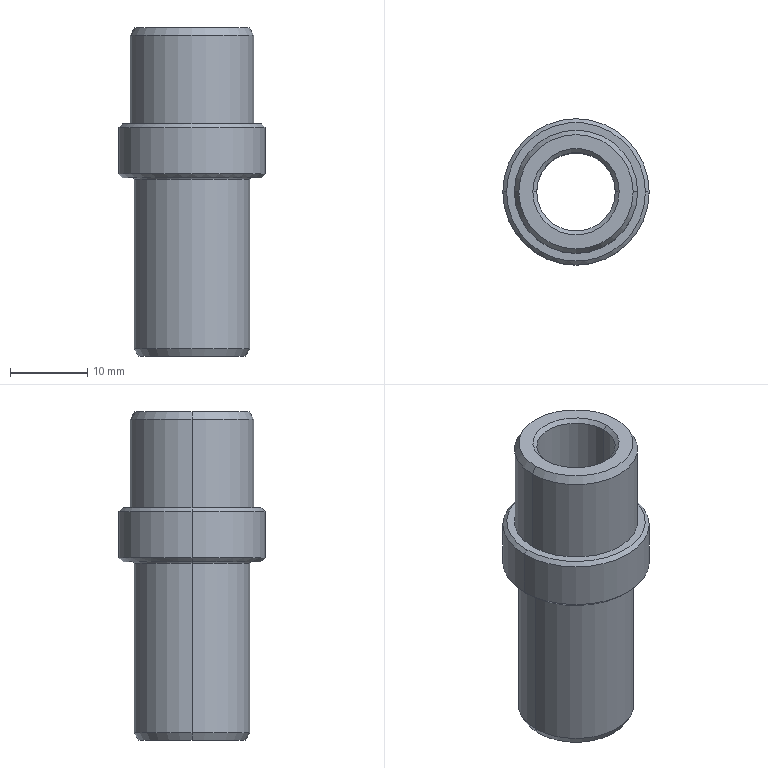Part | STEP file | PERNO RODAJA FRONTAL | 1 solid | 26 faces | box 19 x 19 x 42.7 mm | volume 5059 mm3 | cone 12 | cylinder 8 | plane 4 | torus 2 | commonest cylinder face diameters 10.2 x2 15 x2 16 x2 19 x2
STEP:
#1=CARTESIAN_POINT('',(7.423,0.,10.5));
#2=VERTEX_POINT('',#1);
#3=CARTESIAN_POINT('',(-7.423,0.,10.5));
#4=VERTEX_POINT('',#3);
#5=CARTESIAN_POINT('',(0.,0.,10.5));
#6=DIRECTION('',(0.,0.,1.));
#7=DIRECTION('',(1.,0.,0.));
#8=AXIS2_PLACEMENT_3D('',#5,#6,#7);
#9=CIRCLE('',#8,7.423);
#10=EDGE_CURVE('',#2,#4,#9,.T.);
#11=ORIENTED_EDGE('',*,*,#10,.F.);
#12=CARTESIAN_POINT('',(8.,0.,9.5));
#13=VERTEX_POINT('',#12);
#14=CARTESIAN_POINT('',(7.423,0.,10.5));
#15=DIRECTION('',(0.5,0.,-0.866));
#16=VECTOR('',#15,1000.);
#17=LINE('',#14,#16);
#18=EDGE_CURVE('',#2,#13,#17,.T.);
#19=ORIENTED_EDGE('',*,*,#18,.T.);
#20=CARTESIAN_POINT('',(-8.,0.,9.5));
#21=VERTEX_POINT('',#20);
#22=CARTESIAN_POINT('',(0.,0.,9.5));
#23=DIRECTION('',(0.,0.,-1.));
#24=DIRECTION('',(1.,0.,0.));
#25=AXIS2_PLACEMENT_3D('',#22,#23,#24);
#26=CIRCLE('',#25,8.);
#27=EDGE_CURVE('',#21,#13,#26,.T.);
#28=ORIENTED_EDGE('',*,*,#27,.F.);
#29=CARTESIAN_POINT('',(-7.423,0.,10.5));
#30=DIRECTION('',(-0.5,0.,-0.866));
#31=VECTOR('',#30,1000.);
#32=LINE('',#29,#31);
#33=EDGE_CURVE('',#4,#21,#32,.T.);
#34=ORIENTED_EDGE('',*,*,#33,.F.);
#35=EDGE_LOOP('',(#11,#19,#28,#34));
#36=FACE_OUTER_BOUND('',#35,.T.);
#37=CARTESIAN_POINT('',(0.,0.,10.5));
#38=DIRECTION('',(0.,0.,-1.));
#39=DIRECTION('',(-1.,0.,0.));
#40=AXIS2_PLACEMENT_3D('',#37,#38,#39);
#41=CONICAL_SURFACE('',#40,7.423,0.5236);
#42=ADVANCED_FACE('',(#36),#41,.T.);
#43=CARTESIAN_POINT('',(9.,0.,-2.));
#44=VERTEX_POINT('',#43);
#45=CARTESIAN_POINT('',(-9.,0.,-2.));
#46=VERTEX_POINT('',#45);
#47=CARTESIAN_POINT('',(0.,0.,-2.));
#48=DIRECTION('',(0.,0.,1.));
#49=DIRECTION('',(1.,0.,0.));
#50=AXIS2_PLACEMENT_3D('',#47,#48,#49);
#51=CIRCLE('',#50,9.);
#52=EDGE_CURVE('',#44,#46,#51,.T.);
#53=ORIENTED_EDGE('',*,*,#52,.F.);
#54=CARTESIAN_POINT('',(9.5,0.,-2.5));
#55=VERTEX_POINT('',#54);
#56=CARTESIAN_POINT('',(9.5,0.,-2.5));
#57=DIRECTION('',(0.7071,0.,-0.7071));
#58=VECTOR('',#57,1000.);
#59=LINE('',#56,#58);
#60=EDGE_CURVE('',#44,#55,#59,.T.);
#61=ORIENTED_EDGE('',*,*,#60,.T.);
#62=CARTESIAN_POINT('',(-9.5,0.,-2.5));
#63=VERTEX_POINT('',#62);
#64=CARTESIAN_POINT('',(0.,0.,-2.5));
#65=DIRECTION('',(0.,0.,-1.));
#66=DIRECTION('',(1.,0.,0.));
#67=AXIS2_PLACEMENT_3D('',#64,#65,#66);
#68=CIRCLE('',#67,9.5);
#69=EDGE_CURVE('',#63,#55,#68,.T.);
#70=ORIENTED_EDGE('',*,*,#69,.F.);
#71=CARTESIAN_POINT('',(-9.5,0.,-2.5));
#72=DIRECTION('',(-0.7071,0.,-0.7071));
#73=VECTOR('',#72,1000.);
#74=LINE('',#71,#73);
#75=EDGE_CURVE('',#46,#63,#74,.T.);
#76=ORIENTED_EDGE('',*,*,#75,.F.);
#77=EDGE_LOOP('',(#53,#61,#70,#76));
#78=FACE_OUTER_BOUND('',#77,.T.);
#79=CARTESIAN_POINT('',(0.,0.,-2.5));
#80=DIRECTION('',(0.,0.,-1.));
#81=DIRECTION('',(-1.,0.,0.));
#82=AXIS2_PLACEMENT_3D('',#79,#80,#81);
#83=CONICAL_SURFACE('',#82,9.5,0.7854);
#84=ADVANCED_FACE('',(#78),#83,.T.);
#85=CARTESIAN_POINT('',(-9.,0.,-9.));
#86=VERTEX_POINT('',#85);
#87=CARTESIAN_POINT('',(9.,0.,-9.));
#88=VERTEX_POINT('',#87);
#89=CARTESIAN_POINT('',(0.,0.,-9.));
#90=DIRECTION('',(0.,0.,-1.));
#91=DIRECTION('',(-1.,0.,0.));
#92=AXIS2_PLACEMENT_3D('',#89,#90,#91);
#93=CIRCLE('',#92,9.);
#94=EDGE_CURVE('',#86,#88,#93,.T.);
#95=ORIENTED_EDGE('',*,*,#94,.F.);
#96=CARTESIAN_POINT('',(-9.5,0.,-8.5));
#97=VERTEX_POINT('',#96);
#98=CARTESIAN_POINT('',(-9.,0.,-9.));
#99=DIRECTION('',(-0.7071,0.,0.7071));
#100=VECTOR('',#99,1000.);
#101=LINE('',#98,#100);
#102=EDGE_CURVE('',#86,#97,#101,.T.);
#103=ORIENTED_EDGE('',*,*,#102,.T.);
#104=CARTESIAN_POINT('',(9.5,0.,-8.5));
#105=VERTEX_POINT('',#104);
#106=CARTESIAN_POINT('',(0.,0.,-8.5));
#107=DIRECTION('',(0.,0.,1.));
#108=DIRECTION('',(-1.,0.,0.));
#109=AXIS2_PLACEMENT_3D('',#106,#107,#108);
#110=CIRCLE('',#109,9.5);
#111=EDGE_CURVE('',#105,#97,#110,.T.);
#112=ORIENTED_EDGE('',*,*,#111,.F.);
#113=CARTESIAN_POINT('',(9.,0.,-9.));
#114=DIRECTION('',(0.7071,0.,0.7071));
#115=VECTOR('',#114,1000.);
#116=LINE('',#113,#115);
#117=EDGE_CURVE('',#88,#105,#116,.T.);
#118=ORIENTED_EDGE('',*,*,#117,.F.);
#119=EDGE_LOOP('',(#95,#103,#112,#118));
#120=FACE_OUTER_BOUND('',#119,.T.);
#121=CARTESIAN_POINT('',(0.,0.,-9.));
#122=DIRECTION('',(0.,0.,1.));
#123=DIRECTION('',(1.,0.,0.));
#124=AXIS2_PLACEMENT_3D('',#121,#122,#123);
#125=CONICAL_SURFACE('',#124,9.,0.7854);
#126=ADVANCED_FACE('',(#120),#125,.T.);
#127=CARTESIAN_POINT('',(-5.1,0.,10.));
#128=VERTEX_POINT('',#127);
#129=CARTESIAN_POINT('',(5.1,0.,10.));
#130=VERTEX_POINT('',#129);
#131=CARTESIAN_POINT('',(0.,0.,10.));
#132=DIRECTION('',(0.,0.,1.));
#133=DIRECTION('',(1.,0.,0.));
#134=AXIS2_PLACEMENT_3D('',#131,#132,#133);
#135=CIRCLE('',#134,5.1);
#136=EDGE_CURVE('',#128,#130,#135,.T.);
#137=ORIENTED_EDGE('',*,*,#136,.F.);
#138=CARTESIAN_POINT('',(-5.6,0.,10.5));
#139=VERTEX_POINT('',#138);
#140=CARTESIAN_POINT('',(-5.6,0.,10.5));
#141=DIRECTION('',(-0.7071,0.,0.7071));
#142=VECTOR('',#141,1000.);
#143=LINE('',#140,#142);
#144=EDGE_CURVE('',#128,#139,#143,.T.);
#145=ORIENTED_EDGE('',*,*,#144,.T.);
#146=CARTESIAN_POINT('',(5.6,0.,10.5));
#147=VERTEX_POINT('',#146);
#148=CARTESIAN_POINT('',(0.,0.,10.5));
#149=DIRECTION('',(0.,0.,-1.));
#150=DIRECTION('',(1.,0.,0.));
#151=AXIS2_PLACEMENT_3D('',#148,#149,#150);
#152=CIRCLE('',#151,5.6);
#153=EDGE_CURVE('',#147,#139,#152,.T.);
#154=ORIENTED_EDGE('',*,*,#153,.F.);
#155=CARTESIAN_POINT('',(5.6,0.,10.5));
#156=DIRECTION('',(0.7071,0.,0.7071));
#157=VECTOR('',#156,1000.);
#158=LINE('',#155,#157);
#159=EDGE_CURVE('',#130,#147,#158,.T.);
#160=ORIENTED_EDGE('',*,*,#159,.F.);
#161=EDGE_LOOP('',(#137,#145,#154,#160));
#162=FACE_OUTER_BOUND('',#161,.T.);
#163=CARTESIAN_POINT('',(0.,0.,10.5));
#164=DIRECTION('',(0.,0.,1.));
#165=DIRECTION('',(1.,0.,0.));
#166=AXIS2_PLACEMENT_3D('',#163,#164,#165);
#167=CONICAL_SURFACE('',#166,5.6,0.7854);
#168=ADVANCED_FACE('',(#162),#167,.F.);
#169=CARTESIAN_POINT('',(5.1,0.,-31.7));
#170=VERTEX_POINT('',#169);
#171=CARTESIAN_POINT('',(-5.1,0.,-31.7));
#172=VERTEX_POINT('',#171);
#173=CARTESIAN_POINT('',(0.,0.,-31.7));
#174=DIRECTION('',(0.,0.,-1.));
#175=DIRECTION('',(1.,0.,0.));
#176=AXIS2_PLACEMENT_3D('',#173,#174,#175);
#177=CIRCLE('',#176,5.1);
#178=EDGE_CURVE('',#170,#172,#177,.T.);
#179=ORIENTED_EDGE('',*,*,#178,.F.);
#180=CARTESIAN_POINT('',(5.6,0.,-32.2));
#181=VERTEX_POINT('',#180);
#182=CARTESIAN_POINT('',(5.1,0.,-31.7));
#183=DIRECTION('',(0.7071,0.,-0.7071));
#184=VECTOR('',#183,1000.);
#185=LINE('',#182,#184);
#186=EDGE_CURVE('',#170,#181,#185,.T.);
#187=ORIENTED_EDGE('',*,*,#186,.T.);
#188=CARTESIAN_POINT('',(-5.6,0.,-32.2));
#189=VERTEX_POINT('',#188);
#190=CARTESIAN_POINT('',(0.,0.,-32.2));
#191=DIRECTION('',(0.,0.,1.));
#192=DIRECTION('',(1.,0.,0.));
#193=AXIS2_PLACEMENT_3D('',#190,#191,#192);
#194=CIRCLE('',#193,5.6);
#195=EDGE_CURVE('',#189,#181,#194,.T.);
#196=ORIENTED_EDGE('',*,*,#195,.F.);
#197=CARTESIAN_POINT('',(-5.1,0.,-31.7));
#198=DIRECTION('',(-0.7071,0.,-0.7071));
#199=VECTOR('',#198,1000.);
#200=LINE('',#197,#199);
#201=EDGE_CURVE('',#172,#189,#200,.T.);
#202=ORIENTED_EDGE('',*,*,#201,.F.);
#203=EDGE_LOOP('',(#179,#187,#196,#202));
#204=FACE_OUTER_BOUND('',#203,.T.);
#205=CARTESIAN_POINT('',(0.,0.,-31.7));
#206=DIRECTION('',(0.,0.,-1.));
#207=DIRECTION('',(-1.,0.,0.));
#208=AXIS2_PLACEMENT_3D('',#205,#206,#207);
#209=CONICAL_SURFACE('',#208,5.1,0.7854);
#210=ADVANCED_FACE('',(#204),#209,.F.);
#211=ORIENTED_EDGE('',*,*,#136,.T.);
#212=CARTESIAN_POINT('',(5.1,0.,-32.2));
#213=DIRECTION('',(0.,0.,-1.));
#214=VECTOR('',#213,1000.);
#215=LINE('',#212,#214);
#216=EDGE_CURVE('',#130,#170,#215,.T.);
#217=ORIENTED_EDGE('',*,*,#216,.T.);
#218=ORIENTED_EDGE('',*,*,#178,.T.);
#219=CARTESIAN_POINT('',(-5.1,0.,-32.2));
#220=DIRECTION('',(0.,0.,-1.));
#221=VECTOR('',#220,1000.);
#222=LINE('',#219,#221);
#223=EDGE_CURVE('',#128,#172,#222,.T.);
#224=ORIENTED_EDGE('',*,*,#223,.F.);
#225=EDGE_LOOP('',(#211,#217,#218,#224));
#226=FACE_OUTER_BOUND('',#225,.T.);
#227=CARTESIAN_POINT('',(0.,0.,-32.2));
#228=DIRECTION('',(0.,0.,-1.));
#229=DIRECTION('',(-1.,0.,0.));
#230=AXIS2_PLACEMENT_3D('',#227,#228,#229);
#231=CYLINDRICAL_SURFACE('',#230,5.1);
#232=ADVANCED_FACE('',(#226),#231,.F.);
#233=CARTESIAN_POINT('',(-6.923,0.,-32.2));
#234=VERTEX_POINT('',#233);
#235=CARTESIAN_POINT('',(6.923,0.,-32.2));
#236=VERTEX_POINT('',#235);
#237=CARTESIAN_POINT('',(0.,0.,-32.2));
#238=DIRECTION('',(0.,0.,-1.));
#239=DIRECTION('',(1.,0.,0.));
#240=AXIS2_PLACEMENT_3D('',#237,#238,#239);
#241=CIRCLE('',#240,6.923);
#242=EDGE_CURVE('',#234,#236,#241,.T.);
#243=ORIENTED_EDGE('',*,*,#242,.F.);
#244=CARTESIAN_POINT('',(-7.5,0.,-31.2));
#245=VERTEX_POINT('',#244);
#246=CARTESIAN_POINT('',(-7.5,0.,-31.2));
#247=DIRECTION('',(-0.5,0.,0.866));
#248=VECTOR('',#247,1000.);
#249=LINE('',#246,#248);
#250=EDGE_CURVE('',#234,#245,#249,.T.);
#251=ORIENTED_EDGE('',*,*,#250,.T.);
#252=CARTESIAN_POINT('',(7.5,0.,-31.2));
#253=VERTEX_POINT('',#252);
#254=CARTESIAN_POINT('',(0.,0.,-31.2));
#255=DIRECTION('',(0.,0.,1.));
#256=DIRECTION('',(1.,0.,0.));
#257=AXIS2_PLACEMENT_3D('',#254,#255,#256);
#258=CIRCLE('',#257,7.5);
#259=EDGE_CURVE('',#253,#245,#258,.T.);
#260=ORIENTED_EDGE('',*,*,#259,.F.);
#261=CARTESIAN_POINT('',(7.5,0.,-31.2));
#262=DIRECTION('',(0.5,0.,0.866));
#263=VECTOR('',#262,1000.);
#264=LINE('',#261,#263);
#265=EDGE_CURVE('',#236,#253,#264,.T.);
#266=ORIENTED_EDGE('',*,*,#265,.F.);
#267=EDGE_LOOP('',(#243,#251,#260,#266));
#268=FACE_OUTER_BOUND('',#267,.T.);
#269=CARTESIAN_POINT('',(0.,0.,-31.2));
#270=DIRECTION('',(0.,0.,1.));
#271=DIRECTION('',(1.,0.,0.));
#272=AXIS2_PLACEMENT_3D('',#269,#270,#271);
#273=CONICAL_SURFACE('',#272,7.5,0.5236);
#274=ADVANCED_FACE('',(#268),#273,.T.);
#275=CARTESIAN_POINT('',(7.5,0.,-9.2));
#276=VERTEX_POINT('',#275);
#277=CARTESIAN_POINT('',(-7.5,0.,-9.2));
#278=VERTEX_POINT('',#277);
#279=CARTESIAN_POINT('',(0.,0.,-9.2));
#280=DIRECTION('',(0.,0.,-1.));
#281=DIRECTION('',(-1.,0.,0.));
#282=AXIS2_PLACEMENT_3D('',#279,#280,#281);
#283=CIRCLE('',#282,7.5);
#284=EDGE_CURVE('',#276,#278,#283,.T.);
#285=ORIENTED_EDGE('',*,*,#284,.F.);
#286=CARTESIAN_POINT('',(7.7,0.,-9.));
#287=VERTEX_POINT('',#286);
#288=CARTESIAN_POINT('',(7.7,0.,-9.2));
#289=DIRECTION('',(0.,1.,0.));
#290=DIRECTION('',(-1.,0.,0.));
#291=AXIS2_PLACEMENT_3D('',#288,#289,#290);
#292=CIRCLE('',#291,0.2);
#293=EDGE_CURVE('',#276,#287,#292,.T.);
#294=ORIENTED_EDGE('',*,*,#293,.T.);
#295=CARTESIAN_POINT('',(-7.7,0.,-9.));
#296=VERTEX_POINT('',#295);
#297=CARTESIAN_POINT('',(0.,0.,-9.));
#298=DIRECTION('',(0.,0.,1.));
#299=DIRECTION('',(-1.,0.,0.));
#300=AXIS2_PLACEMENT_3D('',#297,#298,#299);
#301=CIRCLE('',#300,7.7);
#302=EDGE_CURVE('',#296,#287,#301,.T.);
#303=ORIENTED_EDGE('',*,*,#302,.F.);
#304=CARTESIAN_POINT('',(-7.7,0.,-9.2));
#305=DIRECTION('',(0.,-1.,0.));
#306=DIRECTION('',(0.,0.,-1.));
#307=AXIS2_PLACEMENT_3D('',#304,#305,#306);
#308=CIRCLE('',#307,0.2);
#309=EDGE_CURVE('',#278,#296,#308,.T.);
#310=ORIENTED_EDGE('',*,*,#309,.F.);
#311=EDGE_LOOP('',(#285,#294,#303,#310));
#312=FACE_OUTER_BOUND('',#311,.T.);
#313=CARTESIAN_POINT('',(0.,0.,-9.2));
#314=DIRECTION('',(0.,0.,-1.));
#315=DIRECTION('',(-1.,0.,0.));
#316=AXIS2_PLACEMENT_3D('',#313,#314,#315);
#317=TOROIDAL_SURFACE('',#316,7.7,0.2);
#318=ADVANCED_FACE('',(#312),#317,.F.);
#319=ORIENTED_EDGE('',*,*,#259,.T.);
#320=CARTESIAN_POINT('',(-7.5,0.,-32.2));
#321=DIRECTION('',(0.,0.,1.));
#322=VECTOR('',#321,1000.);
#323=LINE('',#320,#322);
#324=EDGE_CURVE('',#245,#278,#323,.T.);
#325=ORIENTED_EDGE('',*,*,#324,.T.);
#326=CARTESIAN_POINT('',(0.,0.,-9.2));
#327=DIRECTION('',(0.,0.,-1.));
#328=DIRECTION('',(-1.,0.,0.));
#329=AXIS2_PLACEMENT_3D('',#326,#327,#328);
#330=CIRCLE('',#329,7.5);
#331=EDGE_CURVE('',#278,#276,#330,.T.);
#332=ORIENTED_EDGE('',*,*,#331,.T.);
#333=CARTESIAN_POINT('',(7.5,0.,-32.2));
#334=DIRECTION('',(0.,0.,1.));
#335=VECTOR('',#334,1000.);
#336=LINE('',#333,#335);
#337=EDGE_CURVE('',#253,#276,#336,.T.);
#338=ORIENTED_EDGE('',*,*,#337,.F.);
#339=EDGE_LOOP('',(#319,#325,#332,#338));
#340=FACE_OUTER_BOUND('',#339,.T.);
#341=CARTESIAN_POINT('',(0.,0.,-32.2));
#342=DIRECTION('',(0.,0.,1.));
#343=DIRECTION('',(1.,0.,0.));
#344=AXIS2_PLACEMENT_3D('',#341,#342,#343);
#345=CYLINDRICAL_SURFACE('',#344,7.5);
#346=ADVANCED_FACE('',(#340),#345,.T.);
#347=ORIENTED_EDGE('',*,*,#69,.T.);
#348=CARTESIAN_POINT('',(9.5,0.,-9.));
#349=DIRECTION('',(0.,0.,-1.));
#350=VECTOR('',#349,1000.);
#351=LINE('',#348,#350);
#352=EDGE_CURVE('',#55,#105,#351,.T.);
#353=ORIENTED_EDGE('',*,*,#352,.T.);
#354=ORIENTED_EDGE('',*,*,#111,.T.);
#355=CARTESIAN_POINT('',(-9.5,0.,-9.));
#356=DIRECTION('',(0.,0.,-1.));
#357=VECTOR('',#356,1000.);
#358=LINE('',#355,#357);
#359=EDGE_CURVE('',#63,#97,#358,.T.);
#360=ORIENTED_EDGE('',*,*,#359,.F.);
#361=EDGE_LOOP('',(#347,#353,#354,#360));
#362=FACE_OUTER_BOUND('',#361,.T.);
#363=CARTESIAN_POINT('',(0.,0.,-9.));
#364=DIRECTION('',(0.,0.,-1.));
#365=DIRECTION('',(-1.,0.,0.));
#366=AXIS2_PLACEMENT_3D('',#363,#364,#365);
#367=CYLINDRICAL_SURFACE('',#366,9.5);
#368=ADVANCED_FACE('',(#362),#367,.T.);
#369=CARTESIAN_POINT('',(-8.,0.,-2.));
#370=VERTEX_POINT('',#369);
#371=CARTESIAN_POINT('',(8.,0.,-2.));
#372=VERTEX_POINT('',#371);
#373=CARTESIAN_POINT('',(0.,0.,-2.));
#374=DIRECTION('',(0.,0.,-1.));
#375=DIRECTION('',(1.,0.,0.));
#376=AXIS2_PLACEMENT_3D('',#373,#374,#375);
#377=CIRCLE('',#376,8.);
#378=EDGE_CURVE('',#370,#372,#377,.T.);
#379=ORIENTED_EDGE('',*,*,#378,.F.);
#380=CARTESIAN_POINT('',(-8.,0.,-32.2));
#381=DIRECTION('',(0.,0.,1.));
#382=VECTOR('',#381,1000.);
#383=LINE('',#380,#382);
#384=EDGE_CURVE('',#370,#21,#383,.T.);
#385=ORIENTED_EDGE('',*,*,#384,.T.);
#386=ORIENTED_EDGE('',*,*,#27,.T.);
#387=CARTESIAN_POINT('',(8.,0.,-32.2));
#388=DIRECTION('',(0.,0.,1.));
#389=VECTOR('',#388,1000.);
#390=LINE('',#387,#389);
#391=EDGE_CURVE('',#372,#13,#390,.T.);
#392=ORIENTED_EDGE('',*,*,#391,.F.);
#393=EDGE_LOOP('',(#379,#385,#386,#392));
#394=FACE_OUTER_BOUND('',#393,.T.);
#395=CARTESIAN_POINT('',(0.,0.,-32.2));
#396=DIRECTION('',(0.,0.,1.));
#397=DIRECTION('',(1.,0.,0.));
#398=AXIS2_PLACEMENT_3D('',#395,#396,#397);
#399=CYLINDRICAL_SURFACE('',#398,8.);
#400=ADVANCED_FACE('',(#394),#399,.T.);
#401=ORIENTED_EDGE('',*,*,#384,.F.);
#402=CARTESIAN_POINT('',(0.,0.,-2.));
#403=DIRECTION('',(0.,0.,-1.));
#404=DIRECTION('',(1.,0.,0.));
#405=AXIS2_PLACEMENT_3D('',#402,#403,#404);
#406=CIRCLE('',#405,8.);
#407=EDGE_CURVE('',#372,#370,#406,.T.);
#408=ORIENTED_EDGE('',*,*,#407,.F.);
#409=ORIENTED_EDGE('',*,*,#391,.T.);
#410=CARTESIAN_POINT('',(0.,0.,9.5));
#411=DIRECTION('',(0.,0.,-1.));
#412=DIRECTION('',(1.,0.,0.));
#413=AXIS2_PLACEMENT_3D('',#410,#411,#412);
#414=CIRCLE('',#413,8.);
#415=EDGE_CURVE('',#13,#21,#414,.T.);
#416=ORIENTED_EDGE('',*,*,#415,.T.);
#417=EDGE_LOOP('',(#401,#408,#409,#416));
#418=FACE_OUTER_BOUND('',#417,.T.);
#419=CARTESIAN_POINT('',(0.,0.,-32.2));
#420=DIRECTION('',(0.,0.,1.));
#421=DIRECTION('',(1.,0.,0.));
#422=AXIS2_PLACEMENT_3D('',#419,#420,#421);
#423=CYLINDRICAL_SURFACE('',#422,8.);
#424=ADVANCED_FACE('',(#418),#423,.T.);
#425=CARTESIAN_POINT('',(0.,0.,10.5));
#426=DIRECTION('',(0.,0.,1.));
#427=DIRECTION('',(1.,0.,0.));
#428=AXIS2_PLACEMENT_3D('',#425,#426,#427);
#429=CIRCLE('',#428,7.423);
#430=EDGE_CURVE('',#4,#2,#429,.T.);
#431=ORIENTED_EDGE('',*,*,#430,.T.);
#432=ORIENTED_EDGE('',*,*,#10,.T.);
#433=EDGE_LOOP('',(#431,#432));
#434=FACE_OUTER_BOUND('',#433,.T.);
#435=ORIENTED_EDGE('',*,*,#153,.T.);
#436=CARTESIAN_POINT('',(0.,0.,10.5));
#437=DIRECTION('',(0.,0.,-1.));
#438=DIRECTION('',(1.,0.,0.));
#439=AXIS2_PLACEMENT_3D('',#436,#437,#438);
#440=CIRCLE('',#439,5.6);
#441=EDGE_CURVE('',#139,#147,#440,.T.);
#442=ORIENTED_EDGE('',*,*,#441,.T.);
#443=EDGE_LOOP('',(#435,#442));
#444=FACE_BOUND('',#443,.T.);
#445=CARTESIAN_POINT('',(0.,0.,10.5));
#446=DIRECTION('',(0.,0.,1.));
#447=DIRECTION('',(1.,0.,0.));
#448=AXIS2_PLACEMENT_3D('',#445,#446,#447);
#449=PLANE('',#448);
#450=ADVANCED_FACE('',(#434,#444),#449,.T.);
#451=CARTESIAN_POINT('',(0.,0.,-2.));
#452=DIRECTION('',(0.,0.,1.));
#453=DIRECTION('',(1.,0.,0.));
#454=AXIS2_PLACEMENT_3D('',#451,#452,#453);
#455=CIRCLE('',#454,9.);
#456=EDGE_CURVE('',#46,#44,#455,.T.);
#457=ORIENTED_EDGE('',*,*,#456,.T.);
#458=ORIENTED_EDGE('',*,*,#52,.T.);
#459=EDGE_LOOP('',(#457,#458));
#460=FACE_OUTER_BOUND('',#459,.T.);
#461=ORIENTED_EDGE('',*,*,#407,.T.);
#462=ORIENTED_EDGE('',*,*,#378,.T.);
#463=EDGE_LOOP('',(#461,#462));
#464=FACE_BOUND('',#463,.T.);
#465=CARTESIAN_POINT('',(0.,0.,-2.));
#466=DIRECTION('',(0.,0.,1.));
#467=DIRECTION('',(1.,0.,0.));
#468=AXIS2_PLACEMENT_3D('',#465,#466,#467);
#469=PLANE('',#468);
#470=ADVANCED_FACE('',(#460,#464),#469,.T.);
#471=ORIENTED_EDGE('',*,*,#352,.F.);
#472=CARTESIAN_POINT('',(0.,0.,-2.5));
#473=DIRECTION('',(0.,0.,-1.));
#474=DIRECTION('',(1.,0.,0.));
#475=AXIS2_PLACEMENT_3D('',#472,#473,#474);
#476=CIRCLE('',#475,9.5);
#477=EDGE_CURVE('',#55,#63,#476,.T.);
#478=ORIENTED_EDGE('',*,*,#477,.T.);
#479=ORIENTED_EDGE('',*,*,#359,.T.);
#480=CARTESIAN_POINT('',(0.,0.,-8.5));
#481=DIRECTION('',(0.,0.,1.));
#482=DIRECTION('',(-1.,0.,0.));
#483=AXIS2_PLACEMENT_3D('',#480,#481,#482);
#484=CIRCLE('',#483,9.5);
#485=EDGE_CURVE('',#97,#105,#484,.T.);
#486=ORIENTED_EDGE('',*,*,#485,.T.);
#487=EDGE_LOOP('',(#471,#478,#479,#486));
#488=FACE_OUTER_BOUND('',#487,.T.);
#489=CARTESIAN_POINT('',(0.,0.,-9.));
#490=DIRECTION('',(0.,0.,-1.));
#491=DIRECTION('',(-1.,0.,0.));
#492=AXIS2_PLACEMENT_3D('',#489,#490,#491);
#493=CYLINDRICAL_SURFACE('',#492,9.5);
#494=ADVANCED_FACE('',(#488),#493,.T.);
#495=CARTESIAN_POINT('',(0.,0.,-9.));
#496=DIRECTION('',(0.,0.,-1.));
#497=DIRECTION('',(-1.,0.,0.));
#498=AXIS2_PLACEMENT_3D('',#495,#496,#497);
#499=CIRCLE('',#498,9.);
#500=EDGE_CURVE('',#88,#86,#499,.T.);
#501=ORIENTED_EDGE('',*,*,#500,.T.);
#502=ORIENTED_EDGE('',*,*,#94,.T.);
#503=EDGE_LOOP('',(#501,#502));
#504=FACE_OUTER_BOUND('',#503,.T.);
#505=ORIENTED_EDGE('',*,*,#302,.T.);
#506=CARTESIAN_POINT('',(0.,0.,-9.));
#507=DIRECTION('',(0.,0.,1.));
#508=DIRECTION('',(-1.,0.,0.));
#509=AXIS2_PLACEMENT_3D('',#506,#507,#508);
#510=CIRCLE('',#509,7.7);
#511=EDGE_CURVE('',#287,#296,#510,.T.);
#512=ORIENTED_EDGE('',*,*,#511,.T.);
#513=EDGE_LOOP('',(#505,#512));
#514=FACE_BOUND('',#513,.T.);
#515=CARTESIAN_POINT('',(0.,9.5,-9.));
#516=DIRECTION('',(0.,0.,-1.));
#517=DIRECTION('',(-1.,0.,0.));
#518=AXIS2_PLACEMENT_3D('',#515,#516,#517);
#519=PLANE('',#518);
#520=ADVANCED_FACE('',(#504,#514),#519,.T.);
#521=ORIENTED_EDGE('',*,*,#195,.T.);
#522=CARTESIAN_POINT('',(0.,0.,-32.2));
#523=DIRECTION('',(0.,0.,1.));
#524=DIRECTION('',(1.,0.,0.));
#525=AXIS2_PLACEMENT_3D('',#522,#523,#524);
#526=CIRCLE('',#525,5.6);
#527=EDGE_CURVE('',#181,#189,#526,.T.);
#528=ORIENTED_EDGE('',*,*,#527,.T.);
#529=EDGE_LOOP('',(#521,#528));
#530=FACE_BOUND('',#529,.T.);
#531=CARTESIAN_POINT('',(0.,0.,-32.2));
#532=DIRECTION('',(0.,0.,-1.));
#533=DIRECTION('',(1.,0.,0.));
#534=AXIS2_PLACEMENT_3D('',#531,#532,#533);
#535=CIRCLE('',#534,6.923);
#536=EDGE_CURVE('',#236,#234,#535,.T.);
#537=ORIENTED_EDGE('',*,*,#536,.T.);
#538=ORIENTED_EDGE('',*,*,#242,.T.);
#539=EDGE_LOOP('',(#537,#538));
#540=FACE_OUTER_BOUND('',#539,.T.);
#541=CARTESIAN_POINT('',(0.,0.,-32.2));
#542=DIRECTION('',(0.,0.,1.));
#543=DIRECTION('',(1.,0.,0.));
#544=AXIS2_PLACEMENT_3D('',#541,#542,#543);
#545=PLANE('',#544);
#546=ADVANCED_FACE('',(#530,#540),#545,.F.);
#547=ORIENTED_EDGE('',*,*,#324,.F.);
#548=CARTESIAN_POINT('',(0.,0.,-31.2));
#549=DIRECTION('',(0.,0.,1.));
#550=DIRECTION('',(1.,0.,0.));
#551=AXIS2_PLACEMENT_3D('',#548,#549,#550);
#552=CIRCLE('',#551,7.5);
#553=EDGE_CURVE('',#245,#253,#552,.T.);
#554=ORIENTED_EDGE('',*,*,#553,.T.);
#555=ORIENTED_EDGE('',*,*,#337,.T.);
#556=ORIENTED_EDGE('',*,*,#284,.T.);
#557=EDGE_LOOP('',(#547,#554,#555,#556));
#558=FACE_OUTER_BOUND('',#557,.T.);
#559=CARTESIAN_POINT('',(0.,0.,-32.2));
#560=DIRECTION('',(0.,0.,1.));
#561=DIRECTION('',(1.,0.,0.));
#562=AXIS2_PLACEMENT_3D('',#559,#560,#561);
#563=CYLINDRICAL_SURFACE('',#562,7.5);
#564=ADVANCED_FACE('',(#558),#563,.T.);
#565=ORIENTED_EDGE('',*,*,#293,.F.);
#566=ORIENTED_EDGE('',*,*,#331,.F.);
#567=ORIENTED_EDGE('',*,*,#309,.T.);
#568=ORIENTED_EDGE('',*,*,#511,.F.);
#569=EDGE_LOOP('',(#565,#566,#567,#568));
#570=FACE_OUTER_BOUND('',#569,.T.);
#571=CARTESIAN_POINT('',(0.,0.,-9.2));
#572=DIRECTION('',(0.,0.,-1.));
#573=DIRECTION('',(-1.,0.,0.));
#574=AXIS2_PLACEMENT_3D('',#571,#572,#573);
#575=TOROIDAL_SURFACE('',#574,7.7,0.2);
#576=ADVANCED_FACE('',(#570),#575,.F.);
#577=ORIENTED_EDGE('',*,*,#250,.F.);
#578=ORIENTED_EDGE('',*,*,#536,.F.);
#579=ORIENTED_EDGE('',*,*,#265,.T.);
#580=ORIENTED_EDGE('',*,*,#553,.F.);
#581=EDGE_LOOP('',(#577,#578,#579,#580));
#582=FACE_OUTER_BOUND('',#581,.T.);
#583=CARTESIAN_POINT('',(0.,0.,-31.2));
#584=DIRECTION('',(0.,0.,1.));
#585=DIRECTION('',(1.,0.,0.));
#586=AXIS2_PLACEMENT_3D('',#583,#584,#585);
#587=CONICAL_SURFACE('',#586,7.5,0.5236);
#588=ADVANCED_FACE('',(#582),#587,.T.);
#589=ORIENTED_EDGE('',*,*,#216,.F.);
#590=CARTESIAN_POINT('',(0.,0.,10.));
#591=DIRECTION('',(0.,0.,1.));
#592=DIRECTION('',(1.,0.,0.));
#593=AXIS2_PLACEMENT_3D('',#590,#591,#592);
#594=CIRCLE('',#593,5.1);
#595=EDGE_CURVE('',#130,#128,#594,.T.);
#596=ORIENTED_EDGE('',*,*,#595,.T.);
#597=ORIENTED_EDGE('',*,*,#223,.T.);
#598=CARTESIAN_POINT('',(0.,0.,-31.7));
#599=DIRECTION('',(0.,0.,-1.));
#600=DIRECTION('',(1.,0.,0.));
#601=AXIS2_PLACEMENT_3D('',#598,#599,#600);
#602=CIRCLE('',#601,5.1);
#603=EDGE_CURVE('',#172,#170,#602,.T.);
#604=ORIENTED_EDGE('',*,*,#603,.T.);
#605=EDGE_LOOP('',(#589,#596,#597,#604));
#606=FACE_OUTER_BOUND('',#605,.T.);
#607=CARTESIAN_POINT('',(0.,0.,-32.2));
#608=DIRECTION('',(0.,0.,-1.));
#609=DIRECTION('',(-1.,0.,0.));
#610=AXIS2_PLACEMENT_3D('',#607,#608,#609);
#611=CYLINDRICAL_SURFACE('',#610,5.1);
#612=ADVANCED_FACE('',(#606),#611,.F.);
#613=ORIENTED_EDGE('',*,*,#186,.F.);
#614=ORIENTED_EDGE('',*,*,#603,.F.);
#615=ORIENTED_EDGE('',*,*,#201,.T.);
#616=ORIENTED_EDGE('',*,*,#527,.F.);
#617=EDGE_LOOP('',(#613,#614,#615,#616));
#618=FACE_OUTER_BOUND('',#617,.T.);
#619=CARTESIAN_POINT('',(0.,0.,-31.7));
#620=DIRECTION('',(0.,0.,-1.));
#621=DIRECTION('',(-1.,0.,0.));
#622=AXIS2_PLACEMENT_3D('',#619,#620,#621);
#623=CONICAL_SURFACE('',#622,5.1,0.7854);
#624=ADVANCED_FACE('',(#618),#623,.F.);
#625=ORIENTED_EDGE('',*,*,#144,.F.);
#626=ORIENTED_EDGE('',*,*,#595,.F.);
#627=ORIENTED_EDGE('',*,*,#159,.T.);
#628=ORIENTED_EDGE('',*,*,#441,.F.);
#629=EDGE_LOOP('',(#625,#626,#627,#628));
#630=FACE_OUTER_BOUND('',#629,.T.);
#631=CARTESIAN_POINT('',(0.,0.,10.5));
#632=DIRECTION('',(0.,0.,1.));
#633=DIRECTION('',(1.,0.,0.));
#634=AXIS2_PLACEMENT_3D('',#631,#632,#633);
#635=CONICAL_SURFACE('',#634,5.6,0.7854);
#636=ADVANCED_FACE('',(#630),#635,.F.);
#637=ORIENTED_EDGE('',*,*,#102,.F.);
#638=ORIENTED_EDGE('',*,*,#500,.F.);
#639=ORIENTED_EDGE('',*,*,#117,.T.);
#640=ORIENTED_EDGE('',*,*,#485,.F.);
#641=EDGE_LOOP('',(#637,#638,#639,#640));
#642=FACE_OUTER_BOUND('',#641,.T.);
#643=CARTESIAN_POINT('',(0.,0.,-9.));
#644=DIRECTION('',(0.,0.,1.));
#645=DIRECTION('',(1.,0.,0.));
#646=AXIS2_PLACEMENT_3D('',#643,#644,#645);
#647=CONICAL_SURFACE('',#646,9.,0.7854);
#648=ADVANCED_FACE('',(#642),#647,.T.);
#649=ORIENTED_EDGE('',*,*,#60,.F.);
#650=ORIENTED_EDGE('',*,*,#456,.F.);
#651=ORIENTED_EDGE('',*,*,#75,.T.);
#652=ORIENTED_EDGE('',*,*,#477,.F.);
#653=EDGE_LOOP('',(#649,#650,#651,#652));
#654=FACE_OUTER_BOUND('',#653,.T.);
#655=CARTESIAN_POINT('',(0.,0.,-2.5));
#656=DIRECTION('',(0.,0.,-1.));
#657=DIRECTION('',(-1.,0.,0.));
#658=AXIS2_PLACEMENT_3D('',#655,#656,#657);
#659=CONICAL_SURFACE('',#658,9.5,0.7854);
#660=ADVANCED_FACE('',(#654),#659,.T.);
#661=ORIENTED_EDGE('',*,*,#18,.F.);
#662=ORIENTED_EDGE('',*,*,#430,.F.);
#663=ORIENTED_EDGE('',*,*,#33,.T.);
#664=ORIENTED_EDGE('',*,*,#415,.F.);
#665=EDGE_LOOP('',(#661,#662,#663,#664));
#666=FACE_OUTER_BOUND('',#665,.T.);
#667=CARTESIAN_POINT('',(0.,0.,10.5));
#668=DIRECTION('',(0.,0.,-1.));
#669=DIRECTION('',(-1.,0.,0.));
#670=AXIS2_PLACEMENT_3D('',#667,#668,#669);
#671=CONICAL_SURFACE('',#670,7.423,0.5236);
#672=ADVANCED_FACE('',(#666),#671,.T.);
#673=CLOSED_SHELL('',(#42,#84,#126,#168,#210,#232,#274,#318,#346,#368,#400,#424,#450,#470,#494,#520,#546,#564,#576,#588,#612,#624,#636,#648,#660,#672));
#674=MANIFOLD_SOLID_BREP('',#673);
#675=CARTESIAN_POINT('',(0.,0.,0.));
#676=DIRECTION('',(0.,0.,1.));
#677=DIRECTION('',(1.,0.,0.));
#678=AXIS2_PLACEMENT_3D('',#675,#676,#677);
#679=(LENGTH_UNIT()NAMED_UNIT(*)SI_UNIT(.MILLI.,.METRE.));
#680=UNCERTAINTY_MEASURE_WITH_UNIT(LENGTH_MEASURE(0.00001),#679,'','');
#681=(NAMED_UNIT(*)PLANE_ANGLE_UNIT()SI_UNIT($,.RADIAN.));
#682=(NAMED_UNIT(*)SI_UNIT($,.STERADIAN.)SOLID_ANGLE_UNIT());
#683=(GEOMETRIC_REPRESENTATION_CONTEXT(3)GLOBAL_UNCERTAINTY_ASSIGNED_CONTEXT((#680))GLOBAL_UNIT_ASSIGNED_CONTEXT((#679,#681,#682))REPRESENTATION_CONTEXT('',''));
#684=ADVANCED_BREP_SHAPE_REPRESENTATION('',(#674,#678),#683);